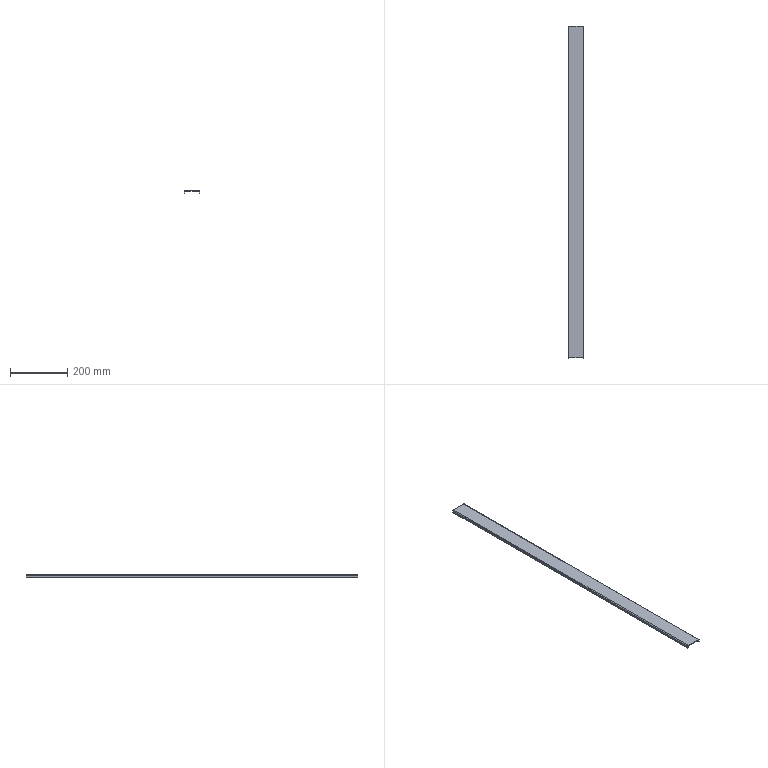Part | SolidWorks | features BaseBody 1 | 1 solid | 22 faces | box 56 x 1162 x 10 mm | volume 201891 mm3 | plane 18 | cylinder 4 | commonest cylinder face diameters 1 x2 6 x2
STEP:
#1=CARTESIAN_POINT('',(-25.5,581.,-10.));
#2=VERTEX_POINT('',#1);
#3=CARTESIAN_POINT('',(-25.5,-581.,-10.));
#4=VERTEX_POINT('',#3);
#5=CARTESIAN_POINT('',(-25.5,-581.,-10.));
#6=DIRECTION('',(0.,-1.,0.));
#7=VECTOR('',#6,1000.);
#8=LINE('',#5,#7);
#9=EDGE_CURVE('',#2,#4,#8,.T.);
#10=ORIENTED_EDGE('',*,*,#9,.T.);
#11=CARTESIAN_POINT('',(-28.,-581.,-10.));
#12=VERTEX_POINT('',#11);
#13=CARTESIAN_POINT('',(-28.,-581.,-10.));
#14=DIRECTION('',(1.,0.,0.));
#15=VECTOR('',#14,1000.);
#16=LINE('',#13,#15);
#17=EDGE_CURVE('',#12,#4,#16,.T.);
#18=ORIENTED_EDGE('',*,*,#17,.F.);
#19=CARTESIAN_POINT('',(-28.,581.,-10.));
#20=VERTEX_POINT('',#19);
#21=CARTESIAN_POINT('',(-28.,0.,-10.));
#22=DIRECTION('',(0.,-1.,0.));
#23=VECTOR('',#22,1000.);
#24=LINE('',#21,#23);
#25=EDGE_CURVE('',#20,#12,#24,.T.);
#26=ORIENTED_EDGE('',*,*,#25,.F.);
#27=CARTESIAN_POINT('',(-28.,581.,-10.));
#28=DIRECTION('',(1.,0.,0.));
#29=VECTOR('',#28,1000.);
#30=LINE('',#27,#29);
#31=EDGE_CURVE('',#20,#2,#30,.T.);
#32=ORIENTED_EDGE('',*,*,#31,.T.);
#33=EDGE_LOOP('',(#10,#18,#26,#32));
#34=FACE_OUTER_BOUND('',#33,.T.);
#35=CARTESIAN_POINT('',(-28.,-581.,-10.));
#36=DIRECTION('',(0.,0.,1.));
#37=DIRECTION('',(1.,0.,0.));
#38=AXIS2_PLACEMENT_3D('',#35,#36,#37);
#39=PLANE('',#38);
#40=ADVANCED_FACE('',(#34),#39,.F.);
#41=CARTESIAN_POINT('',(-25.5,581.,-3.));
#42=VERTEX_POINT('',#41);
#43=CARTESIAN_POINT('',(-25.5,581.,-10.));
#44=DIRECTION('',(0.,0.,-1.));
#45=VECTOR('',#44,1000.);
#46=LINE('',#43,#45);
#47=EDGE_CURVE('',#42,#2,#46,.T.);
#48=ORIENTED_EDGE('',*,*,#47,.F.);
#49=CARTESIAN_POINT('',(-25.5,-581.,-3.));
#50=VERTEX_POINT('',#49);
#51=CARTESIAN_POINT('',(-25.5,-581.,-3.));
#52=DIRECTION('',(0.,1.,0.));
#53=VECTOR('',#52,1000.);
#54=LINE('',#51,#53);
#55=EDGE_CURVE('',#50,#42,#54,.T.);
#56=ORIENTED_EDGE('',*,*,#55,.F.);
#57=CARTESIAN_POINT('',(-25.5,-581.,-2.5));
#58=DIRECTION('',(0.,0.,1.));
#59=VECTOR('',#58,1000.);
#60=LINE('',#57,#59);
#61=EDGE_CURVE('',#4,#50,#60,.T.);
#62=ORIENTED_EDGE('',*,*,#61,.F.);
#63=ORIENTED_EDGE('',*,*,#9,.F.);
#64=EDGE_LOOP('',(#48,#56,#62,#63));
#65=FACE_OUTER_BOUND('',#64,.T.);
#66=CARTESIAN_POINT('',(-25.5,0.,0.));
#67=DIRECTION('',(1.,0.,0.));
#68=DIRECTION('',(0.,0.,-1.));
#69=AXIS2_PLACEMENT_3D('',#66,#67,#68);
#70=PLANE('',#69);
#71=ADVANCED_FACE('',(#65),#70,.T.);
#72=CARTESIAN_POINT('',(-28.,581.,-3.));
#73=VERTEX_POINT('',#72);
#74=CARTESIAN_POINT('',(-28.,-581.,-3.));
#75=VERTEX_POINT('',#74);
#76=CARTESIAN_POINT('',(-28.,-581.,-3.));
#77=DIRECTION('',(0.,-1.,0.));
#78=VECTOR('',#77,1000.);
#79=LINE('',#76,#78);
#80=EDGE_CURVE('',#73,#75,#79,.T.);
#81=ORIENTED_EDGE('',*,*,#80,.F.);
#82=CARTESIAN_POINT('',(-28.,581.,0.));
#83=DIRECTION('',(0.,0.,-1.));
#84=VECTOR('',#83,1000.);
#85=LINE('',#82,#84);
#86=EDGE_CURVE('',#73,#20,#85,.T.);
#87=ORIENTED_EDGE('',*,*,#86,.T.);
#88=ORIENTED_EDGE('',*,*,#25,.T.);
#89=CARTESIAN_POINT('',(-28.,-581.,0.));
#90=DIRECTION('',(0.,0.,1.));
#91=VECTOR('',#90,1000.);
#92=LINE('',#89,#91);
#93=EDGE_CURVE('',#12,#75,#92,.T.);
#94=ORIENTED_EDGE('',*,*,#93,.T.);
#95=EDGE_LOOP('',(#81,#87,#88,#94));
#96=FACE_OUTER_BOUND('',#95,.T.);
#97=CARTESIAN_POINT('',(-28.,0.,0.));
#98=DIRECTION('',(1.,0.,0.));
#99=DIRECTION('',(0.,0.,-1.));
#100=AXIS2_PLACEMENT_3D('',#97,#98,#99);
#101=PLANE('',#100);
#102=ADVANCED_FACE('',(#96),#101,.F.);
#103=CARTESIAN_POINT('',(-28.,-581.,-3.));
#104=DIRECTION('',(-1.,0.,0.));
#105=VECTOR('',#104,1000.);
#106=LINE('',#103,#105);
#107=EDGE_CURVE('',#50,#75,#106,.T.);
#108=ORIENTED_EDGE('',*,*,#107,.T.);
#109=ORIENTED_EDGE('',*,*,#93,.F.);
#110=ORIENTED_EDGE('',*,*,#17,.T.);
#111=ORIENTED_EDGE('',*,*,#61,.T.);
#112=EDGE_LOOP('',(#108,#109,#110,#111));
#113=FACE_OUTER_BOUND('',#112,.T.);
#114=CARTESIAN_POINT('',(-28.,-581.,-2.5));
#115=DIRECTION('',(0.,1.,0.));
#116=DIRECTION('',(1.,0.,0.));
#117=AXIS2_PLACEMENT_3D('',#114,#115,#116);
#118=PLANE('',#117);
#119=ADVANCED_FACE('',(#113),#118,.F.);
#120=CARTESIAN_POINT('',(-25.5,581.,-3.));
#121=DIRECTION('',(-1.,0.,0.));
#122=VECTOR('',#121,1000.);
#123=LINE('',#120,#122);
#124=EDGE_CURVE('',#42,#73,#123,.T.);
#125=ORIENTED_EDGE('',*,*,#124,.F.);
#126=ORIENTED_EDGE('',*,*,#47,.T.);
#127=ORIENTED_EDGE('',*,*,#31,.F.);
#128=ORIENTED_EDGE('',*,*,#86,.F.);
#129=EDGE_LOOP('',(#125,#126,#127,#128));
#130=FACE_OUTER_BOUND('',#129,.T.);
#131=CARTESIAN_POINT('',(-28.,581.,-10.));
#132=DIRECTION('',(0.,-1.,0.));
#133=DIRECTION('',(0.,0.,-1.));
#134=AXIS2_PLACEMENT_3D('',#131,#132,#133);
#135=PLANE('',#134);
#136=ADVANCED_FACE('',(#130),#135,.F.);
#137=CARTESIAN_POINT('',(-25.,581.,-2.5));
#138=VERTEX_POINT('',#137);
#139=CARTESIAN_POINT('',(-25.,-581.,-2.5));
#140=VERTEX_POINT('',#139);
#141=CARTESIAN_POINT('',(-25.,581.,-2.5));
#142=DIRECTION('',(0.,-1.,0.));
#143=VECTOR('',#142,1000.);
#144=LINE('',#141,#143);
#145=EDGE_CURVE('',#138,#140,#144,.T.);
#146=ORIENTED_EDGE('',*,*,#145,.T.);
#147=CARTESIAN_POINT('',(-25.,-581.,-3.));
#148=DIRECTION('',(0.,-1.,0.));
#149=DIRECTION('',(0.,0.,1.));
#150=AXIS2_PLACEMENT_3D('',#147,#148,#149);
#151=CIRCLE('',#150,0.5);
#152=EDGE_CURVE('',#140,#50,#151,.T.);
#153=ORIENTED_EDGE('',*,*,#152,.T.);
#154=ORIENTED_EDGE('',*,*,#55,.T.);
#155=CARTESIAN_POINT('',(-25.,581.,-3.));
#156=DIRECTION('',(0.,1.,0.));
#157=DIRECTION('',(0.,0.,1.));
#158=AXIS2_PLACEMENT_3D('',#155,#156,#157);
#159=CIRCLE('',#158,0.5);
#160=EDGE_CURVE('',#42,#138,#159,.T.);
#161=ORIENTED_EDGE('',*,*,#160,.T.);
#162=EDGE_LOOP('',(#146,#153,#154,#161));
#163=FACE_OUTER_BOUND('',#162,.T.);
#164=CARTESIAN_POINT('',(-25.,581.,-3.));
#165=DIRECTION('',(0.,1.,0.));
#166=DIRECTION('',(-1.,0.,0.));
#167=AXIS2_PLACEMENT_3D('',#164,#165,#166);
#168=CYLINDRICAL_SURFACE('',#167,0.5);
#169=ADVANCED_FACE('',(#163),#168,.F.);
#170=CARTESIAN_POINT('',(-25.,581.,0.));
#171=VERTEX_POINT('',#170);
#172=CARTESIAN_POINT('',(-25.,-581.,0.));
#173=VERTEX_POINT('',#172);
#174=CARTESIAN_POINT('',(-25.,581.,0.));
#175=DIRECTION('',(0.,-1.,0.));
#176=VECTOR('',#175,1000.);
#177=LINE('',#174,#176);
#178=EDGE_CURVE('',#171,#173,#177,.T.);
#179=ORIENTED_EDGE('',*,*,#178,.F.);
#180=CARTESIAN_POINT('',(-25.,581.,-3.));
#181=DIRECTION('',(0.,1.,0.));
#182=DIRECTION('',(0.,0.,1.));
#183=AXIS2_PLACEMENT_3D('',#180,#181,#182);
#184=CIRCLE('',#183,3.);
#185=EDGE_CURVE('',#73,#171,#184,.T.);
#186=ORIENTED_EDGE('',*,*,#185,.F.);
#187=ORIENTED_EDGE('',*,*,#80,.T.);
#188=CARTESIAN_POINT('',(-25.,-581.,-3.));
#189=DIRECTION('',(0.,-1.,0.));
#190=DIRECTION('',(0.,0.,1.));
#191=AXIS2_PLACEMENT_3D('',#188,#189,#190);
#192=CIRCLE('',#191,3.);
#193=EDGE_CURVE('',#173,#75,#192,.T.);
#194=ORIENTED_EDGE('',*,*,#193,.F.);
#195=EDGE_LOOP('',(#179,#186,#187,#194));
#196=FACE_OUTER_BOUND('',#195,.T.);
#197=CARTESIAN_POINT('',(-25.,581.,-3.));
#198=DIRECTION('',(0.,1.,0.));
#199=DIRECTION('',(-1.,0.,0.));
#200=AXIS2_PLACEMENT_3D('',#197,#198,#199);
#201=CYLINDRICAL_SURFACE('',#200,3.);
#202=ADVANCED_FACE('',(#196),#201,.T.);
#203=ORIENTED_EDGE('',*,*,#160,.F.);
#204=ORIENTED_EDGE('',*,*,#124,.T.);
#205=ORIENTED_EDGE('',*,*,#185,.T.);
#206=CARTESIAN_POINT('',(-25.,581.,-2.5));
#207=DIRECTION('',(0.,0.,1.));
#208=VECTOR('',#207,1000.);
#209=LINE('',#206,#208);
#210=EDGE_CURVE('',#138,#171,#209,.T.);
#211=ORIENTED_EDGE('',*,*,#210,.F.);
#212=EDGE_LOOP('',(#203,#204,#205,#211));
#213=FACE_OUTER_BOUND('',#212,.T.);
#214=CARTESIAN_POINT('',(-25.,581.,-3.));
#215=DIRECTION('',(0.,-1.,0.));
#216=DIRECTION('',(0.,0.,-1.));
#217=AXIS2_PLACEMENT_3D('',#214,#215,#216);
#218=PLANE('',#217);
#219=ADVANCED_FACE('',(#213),#218,.F.);
#220=ORIENTED_EDGE('',*,*,#107,.F.);
#221=ORIENTED_EDGE('',*,*,#152,.F.);
#222=CARTESIAN_POINT('',(-25.,-581.,-2.5));
#223=DIRECTION('',(0.,0.,1.));
#224=VECTOR('',#223,1000.);
#225=LINE('',#222,#224);
#226=EDGE_CURVE('',#140,#173,#225,.T.);
#227=ORIENTED_EDGE('',*,*,#226,.T.);
#228=ORIENTED_EDGE('',*,*,#193,.T.);
#229=EDGE_LOOP('',(#220,#221,#227,#228));
#230=FACE_OUTER_BOUND('',#229,.T.);
#231=CARTESIAN_POINT('',(-25.,-581.,-3.));
#232=DIRECTION('',(0.,-1.,0.));
#233=DIRECTION('',(0.,0.,-1.));
#234=AXIS2_PLACEMENT_3D('',#231,#232,#233);
#235=PLANE('',#234);
#236=ADVANCED_FACE('',(#230),#235,.T.);
#237=CARTESIAN_POINT('',(25.5,-581.,-10.));
#238=VERTEX_POINT('',#237);
#239=CARTESIAN_POINT('',(25.5,581.,-10.));
#240=VERTEX_POINT('',#239);
#241=CARTESIAN_POINT('',(25.5,581.,-10.));
#242=DIRECTION('',(0.,1.,0.));
#243=VECTOR('',#242,1000.);
#244=LINE('',#241,#243);
#245=EDGE_CURVE('',#238,#240,#244,.T.);
#246=ORIENTED_EDGE('',*,*,#245,.T.);
#247=CARTESIAN_POINT('',(28.,581.,-10.));
#248=VERTEX_POINT('',#247);
#249=CARTESIAN_POINT('',(28.,581.,-10.));
#250=DIRECTION('',(-1.,0.,0.));
#251=VECTOR('',#250,1000.);
#252=LINE('',#249,#251);
#253=EDGE_CURVE('',#248,#240,#252,.T.);
#254=ORIENTED_EDGE('',*,*,#253,.F.);
#255=CARTESIAN_POINT('',(28.,-581.,-10.));
#256=VERTEX_POINT('',#255);
#257=CARTESIAN_POINT('',(28.,0.,-10.));
#258=DIRECTION('',(0.,1.,0.));
#259=VECTOR('',#258,1000.);
#260=LINE('',#257,#259);
#261=EDGE_CURVE('',#256,#248,#260,.T.);
#262=ORIENTED_EDGE('',*,*,#261,.F.);
#263=CARTESIAN_POINT('',(28.,-581.,-10.));
#264=DIRECTION('',(-1.,0.,0.));
#265=VECTOR('',#264,1000.);
#266=LINE('',#263,#265);
#267=EDGE_CURVE('',#256,#238,#266,.T.);
#268=ORIENTED_EDGE('',*,*,#267,.T.);
#269=EDGE_LOOP('',(#246,#254,#262,#268));
#270=FACE_OUTER_BOUND('',#269,.T.);
#271=CARTESIAN_POINT('',(28.,581.,-10.));
#272=DIRECTION('',(0.,0.,1.));
#273=DIRECTION('',(1.,0.,0.));
#274=AXIS2_PLACEMENT_3D('',#271,#272,#273);
#275=PLANE('',#274);
#276=ADVANCED_FACE('',(#270),#275,.F.);
#277=CARTESIAN_POINT('',(25.5,-581.,-3.));
#278=VERTEX_POINT('',#277);
#279=CARTESIAN_POINT('',(25.5,-581.,-10.));
#280=DIRECTION('',(0.,0.,-1.));
#281=VECTOR('',#280,1000.);
#282=LINE('',#279,#281);
#283=EDGE_CURVE('',#278,#238,#282,.T.);
#284=ORIENTED_EDGE('',*,*,#283,.F.);
#285=CARTESIAN_POINT('',(25.5,581.,-3.));
#286=VERTEX_POINT('',#285);
#287=CARTESIAN_POINT('',(25.5,581.,-3.));
#288=DIRECTION('',(0.,-1.,0.));
#289=VECTOR('',#288,1000.);
#290=LINE('',#287,#289);
#291=EDGE_CURVE('',#286,#278,#290,.T.);
#292=ORIENTED_EDGE('',*,*,#291,.F.);
#293=CARTESIAN_POINT('',(25.5,581.,-2.5));
#294=DIRECTION('',(0.,0.,1.));
#295=VECTOR('',#294,1000.);
#296=LINE('',#293,#295);
#297=EDGE_CURVE('',#240,#286,#296,.T.);
#298=ORIENTED_EDGE('',*,*,#297,.F.);
#299=ORIENTED_EDGE('',*,*,#245,.F.);
#300=EDGE_LOOP('',(#284,#292,#298,#299));
#301=FACE_OUTER_BOUND('',#300,.T.);
#302=CARTESIAN_POINT('',(25.5,0.,0.));
#303=DIRECTION('',(-1.,0.,0.));
#304=DIRECTION('',(0.,0.,1.));
#305=AXIS2_PLACEMENT_3D('',#302,#303,#304);
#306=PLANE('',#305);
#307=ADVANCED_FACE('',(#301),#306,.T.);
#308=CARTESIAN_POINT('',(28.,-581.,-3.));
#309=VERTEX_POINT('',#308);
#310=CARTESIAN_POINT('',(28.,581.,-3.));
#311=VERTEX_POINT('',#310);
#312=CARTESIAN_POINT('',(28.,581.,-3.));
#313=DIRECTION('',(0.,1.,0.));
#314=VECTOR('',#313,1000.);
#315=LINE('',#312,#314);
#316=EDGE_CURVE('',#309,#311,#315,.T.);
#317=ORIENTED_EDGE('',*,*,#316,.F.);
#318=CARTESIAN_POINT('',(28.,-581.,0.));
#319=DIRECTION('',(0.,0.,-1.));
#320=VECTOR('',#319,1000.);
#321=LINE('',#318,#320);
#322=EDGE_CURVE('',#309,#256,#321,.T.);
#323=ORIENTED_EDGE('',*,*,#322,.T.);
#324=ORIENTED_EDGE('',*,*,#261,.T.);
#325=CARTESIAN_POINT('',(28.,581.,0.));
#326=DIRECTION('',(0.,0.,1.));
#327=VECTOR('',#326,1000.);
#328=LINE('',#325,#327);
#329=EDGE_CURVE('',#248,#311,#328,.T.);
#330=ORIENTED_EDGE('',*,*,#329,.T.);
#331=EDGE_LOOP('',(#317,#323,#324,#330));
#332=FACE_OUTER_BOUND('',#331,.T.);
#333=CARTESIAN_POINT('',(28.,0.,0.));
#334=DIRECTION('',(-1.,0.,0.));
#335=DIRECTION('',(0.,0.,1.));
#336=AXIS2_PLACEMENT_3D('',#333,#334,#335);
#337=PLANE('',#336);
#338=ADVANCED_FACE('',(#332),#337,.F.);
#339=CARTESIAN_POINT('',(28.,581.,-3.));
#340=DIRECTION('',(1.,0.,0.));
#341=VECTOR('',#340,1000.);
#342=LINE('',#339,#341);
#343=EDGE_CURVE('',#286,#311,#342,.T.);
#344=ORIENTED_EDGE('',*,*,#343,.T.);
#345=ORIENTED_EDGE('',*,*,#329,.F.);
#346=ORIENTED_EDGE('',*,*,#253,.T.);
#347=ORIENTED_EDGE('',*,*,#297,.T.);
#348=EDGE_LOOP('',(#344,#345,#346,#347));
#349=FACE_OUTER_BOUND('',#348,.T.);
#350=CARTESIAN_POINT('',(28.,581.,-2.5));
#351=DIRECTION('',(0.,-1.,0.));
#352=DIRECTION('',(0.,0.,-1.));
#353=AXIS2_PLACEMENT_3D('',#350,#351,#352);
#354=PLANE('',#353);
#355=ADVANCED_FACE('',(#349),#354,.F.);
#356=CARTESIAN_POINT('',(25.5,-581.,-3.));
#357=DIRECTION('',(1.,0.,0.));
#358=VECTOR('',#357,1000.);
#359=LINE('',#356,#358);
#360=EDGE_CURVE('',#278,#309,#359,.T.);
#361=ORIENTED_EDGE('',*,*,#360,.F.);
#362=ORIENTED_EDGE('',*,*,#283,.T.);
#363=ORIENTED_EDGE('',*,*,#267,.F.);
#364=ORIENTED_EDGE('',*,*,#322,.F.);
#365=EDGE_LOOP('',(#361,#362,#363,#364));
#366=FACE_OUTER_BOUND('',#365,.T.);
#367=CARTESIAN_POINT('',(28.,-581.,-10.));
#368=DIRECTION('',(0.,1.,0.));
#369=DIRECTION('',(1.,0.,0.));
#370=AXIS2_PLACEMENT_3D('',#367,#368,#369);
#371=PLANE('',#370);
#372=ADVANCED_FACE('',(#366),#371,.F.);
#373=CARTESIAN_POINT('',(25.,-581.,-2.5));
#374=VERTEX_POINT('',#373);
#375=CARTESIAN_POINT('',(25.,581.,-2.5));
#376=VERTEX_POINT('',#375);
#377=CARTESIAN_POINT('',(25.,-581.,-2.5));
#378=DIRECTION('',(0.,1.,0.));
#379=VECTOR('',#378,1000.);
#380=LINE('',#377,#379);
#381=EDGE_CURVE('',#374,#376,#380,.T.);
#382=ORIENTED_EDGE('',*,*,#381,.T.);
#383=CARTESIAN_POINT('',(25.,581.,-3.));
#384=DIRECTION('',(0.,1.,0.));
#385=DIRECTION('',(0.,0.,-1.));
#386=AXIS2_PLACEMENT_3D('',#383,#384,#385);
#387=CIRCLE('',#386,0.5);
#388=EDGE_CURVE('',#376,#286,#387,.T.);
#389=ORIENTED_EDGE('',*,*,#388,.T.);
#390=ORIENTED_EDGE('',*,*,#291,.T.);
#391=CARTESIAN_POINT('',(25.,-581.,-3.));
#392=DIRECTION('',(0.,-1.,0.));
#393=DIRECTION('',(0.,0.,-1.));
#394=AXIS2_PLACEMENT_3D('',#391,#392,#393);
#395=CIRCLE('',#394,0.5);
#396=EDGE_CURVE('',#278,#374,#395,.T.);
#397=ORIENTED_EDGE('',*,*,#396,.T.);
#398=EDGE_LOOP('',(#382,#389,#390,#397));
#399=FACE_OUTER_BOUND('',#398,.T.);
#400=CARTESIAN_POINT('',(25.,-581.,-3.));
#401=DIRECTION('',(0.,-1.,0.));
#402=DIRECTION('',(1.,0.,0.));
#403=AXIS2_PLACEMENT_3D('',#400,#401,#402);
#404=CYLINDRICAL_SURFACE('',#403,0.5);
#405=ADVANCED_FACE('',(#399),#404,.F.);
#406=CARTESIAN_POINT('',(25.,-581.,0.));
#407=VERTEX_POINT('',#406);
#408=CARTESIAN_POINT('',(25.,581.,0.));
#409=VERTEX_POINT('',#408);
#410=CARTESIAN_POINT('',(25.,-581.,0.));
#411=DIRECTION('',(0.,1.,0.));
#412=VECTOR('',#411,1000.);
#413=LINE('',#410,#412);
#414=EDGE_CURVE('',#407,#409,#413,.T.);
#415=ORIENTED_EDGE('',*,*,#414,.F.);
#416=CARTESIAN_POINT('',(25.,-581.,-3.));
#417=DIRECTION('',(0.,-1.,0.));
#418=DIRECTION('',(0.,0.,-1.));
#419=AXIS2_PLACEMENT_3D('',#416,#417,#418);
#420=CIRCLE('',#419,3.);
#421=EDGE_CURVE('',#309,#407,#420,.T.);
#422=ORIENTED_EDGE('',*,*,#421,.F.);
#423=ORIENTED_EDGE('',*,*,#316,.T.);
#424=CARTESIAN_POINT('',(25.,581.,-3.));
#425=DIRECTION('',(0.,1.,0.));
#426=DIRECTION('',(0.,0.,-1.));
#427=AXIS2_PLACEMENT_3D('',#424,#425,#426);
#428=CIRCLE('',#427,3.);
#429=EDGE_CURVE('',#409,#311,#428,.T.);
#430=ORIENTED_EDGE('',*,*,#429,.F.);
#431=EDGE_LOOP('',(#415,#422,#423,#430));
#432=FACE_OUTER_BOUND('',#431,.T.);
#433=CARTESIAN_POINT('',(25.,-581.,-3.));
#434=DIRECTION('',(0.,-1.,0.));
#435=DIRECTION('',(1.,0.,0.));
#436=AXIS2_PLACEMENT_3D('',#433,#434,#435);
#437=CYLINDRICAL_SURFACE('',#436,3.);
#438=ADVANCED_FACE('',(#432),#437,.T.);
#439=ORIENTED_EDGE('',*,*,#396,.F.);
#440=ORIENTED_EDGE('',*,*,#360,.T.);
#441=ORIENTED_EDGE('',*,*,#421,.T.);
#442=CARTESIAN_POINT('',(25.,-581.,-2.5));
#443=DIRECTION('',(0.,0.,1.));
#444=VECTOR('',#443,1000.);
#445=LINE('',#442,#444);
#446=EDGE_CURVE('',#374,#407,#445,.T.);
#447=ORIENTED_EDGE('',*,*,#446,.F.);
#448=EDGE_LOOP('',(#439,#440,#441,#447));
#449=FACE_OUTER_BOUND('',#448,.T.);
#450=CARTESIAN_POINT('',(25.,-581.,-3.));
#451=DIRECTION('',(0.,1.,0.));
#452=DIRECTION('',(1.,0.,0.));
#453=AXIS2_PLACEMENT_3D('',#450,#451,#452);
#454=PLANE('',#453);
#455=ADVANCED_FACE('',(#449),#454,.F.);
#456=ORIENTED_EDGE('',*,*,#343,.F.);
#457=ORIENTED_EDGE('',*,*,#388,.F.);
#458=CARTESIAN_POINT('',(25.,581.,-2.5));
#459=DIRECTION('',(0.,0.,1.));
#460=VECTOR('',#459,1000.);
#461=LINE('',#458,#460);
#462=EDGE_CURVE('',#376,#409,#461,.T.);
#463=ORIENTED_EDGE('',*,*,#462,.T.);
#464=ORIENTED_EDGE('',*,*,#429,.T.);
#465=EDGE_LOOP('',(#456,#457,#463,#464));
#466=FACE_OUTER_BOUND('',#465,.T.);
#467=CARTESIAN_POINT('',(25.,581.,-3.));
#468=DIRECTION('',(0.,1.,0.));
#469=DIRECTION('',(1.,0.,0.));
#470=AXIS2_PLACEMENT_3D('',#467,#468,#469);
#471=PLANE('',#470);
#472=ADVANCED_FACE('',(#466),#471,.T.);
#473=ORIENTED_EDGE('',*,*,#226,.F.);
#474=CARTESIAN_POINT('',(28.,-581.,-2.5));
#475=DIRECTION('',(1.,0.,0.));
#476=VECTOR('',#475,1000.);
#477=LINE('',#474,#476);
#478=EDGE_CURVE('',#140,#374,#477,.T.);
#479=ORIENTED_EDGE('',*,*,#478,.T.);
#480=ORIENTED_EDGE('',*,*,#446,.T.);
#481=CARTESIAN_POINT('',(28.,-581.,0.));
#482=DIRECTION('',(1.,0.,0.));
#483=VECTOR('',#482,1000.);
#484=LINE('',#481,#483);
#485=EDGE_CURVE('',#173,#407,#484,.T.);
#486=ORIENTED_EDGE('',*,*,#485,.F.);
#487=EDGE_LOOP('',(#473,#479,#480,#486));
#488=FACE_OUTER_BOUND('',#487,.T.);
#489=CARTESIAN_POINT('',(28.,-581.,-2.5));
#490=DIRECTION('',(0.,-1.,0.));
#491=DIRECTION('',(0.,0.,-1.));
#492=AXIS2_PLACEMENT_3D('',#489,#490,#491);
#493=PLANE('',#492);
#494=ADVANCED_FACE('',(#488),#493,.T.);
#495=CARTESIAN_POINT('',(28.,581.,-2.5));
#496=DIRECTION('',(-1.,0.,0.));
#497=VECTOR('',#496,1000.);
#498=LINE('',#495,#497);
#499=EDGE_CURVE('',#376,#138,#498,.T.);
#500=ORIENTED_EDGE('',*,*,#499,.T.);
#501=ORIENTED_EDGE('',*,*,#210,.T.);
#502=CARTESIAN_POINT('',(28.,581.,0.));
#503=DIRECTION('',(-1.,0.,0.));
#504=VECTOR('',#503,1000.);
#505=LINE('',#502,#504);
#506=EDGE_CURVE('',#409,#171,#505,.T.);
#507=ORIENTED_EDGE('',*,*,#506,.F.);
#508=ORIENTED_EDGE('',*,*,#462,.F.);
#509=EDGE_LOOP('',(#500,#501,#507,#508));
#510=FACE_OUTER_BOUND('',#509,.T.);
#511=CARTESIAN_POINT('',(28.,581.,-2.5));
#512=DIRECTION('',(0.,1.,0.));
#513=DIRECTION('',(1.,0.,0.));
#514=AXIS2_PLACEMENT_3D('',#511,#512,#513);
#515=PLANE('',#514);
#516=ADVANCED_FACE('',(#510),#515,.T.);
#517=ORIENTED_EDGE('',*,*,#178,.T.);
#518=ORIENTED_EDGE('',*,*,#485,.T.);
#519=ORIENTED_EDGE('',*,*,#414,.T.);
#520=ORIENTED_EDGE('',*,*,#506,.T.);
#521=EDGE_LOOP('',(#517,#518,#519,#520));
#522=FACE_OUTER_BOUND('',#521,.T.);
#523=CARTESIAN_POINT('',(0.,0.,0.));
#524=DIRECTION('',(0.,0.,-1.));
#525=DIRECTION('',(0.,-1.,0.));
#526=AXIS2_PLACEMENT_3D('',#523,#524,#525);
#527=PLANE('',#526);
#528=ADVANCED_FACE('',(#522),#527,.F.);
#529=ORIENTED_EDGE('',*,*,#478,.F.);
#530=ORIENTED_EDGE('',*,*,#145,.F.);
#531=ORIENTED_EDGE('',*,*,#499,.F.);
#532=ORIENTED_EDGE('',*,*,#381,.F.);
#533=EDGE_LOOP('',(#529,#530,#531,#532));
#534=FACE_OUTER_BOUND('',#533,.T.);
#535=CARTESIAN_POINT('',(0.,0.,-2.5));
#536=DIRECTION('',(0.,0.,-1.));
#537=DIRECTION('',(0.,-1.,0.));
#538=AXIS2_PLACEMENT_3D('',#535,#536,#537);
#539=PLANE('',#538);
#540=ADVANCED_FACE('',(#534),#539,.T.);
#541=CLOSED_SHELL('',(#40,#71,#102,#119,#136,#169,#202,#219,#236,#276,#307,#338,#355,#372,#405,#438,#455,#472,#494,#516,#528,#540));
#542=MANIFOLD_SOLID_BREP('',#541);
#543=CARTESIAN_POINT('',(0.,0.,0.));
#544=DIRECTION('',(0.,0.,1.));
#545=DIRECTION('',(1.,0.,0.));
#546=AXIS2_PLACEMENT_3D('',#543,#544,#545);
#547=(LENGTH_UNIT()NAMED_UNIT(*)SI_UNIT(.MILLI.,.METRE.));
#548=UNCERTAINTY_MEASURE_WITH_UNIT(LENGTH_MEASURE(0.00001),#547,'','');
#549=(NAMED_UNIT(*)PLANE_ANGLE_UNIT()SI_UNIT($,.RADIAN.));
#550=(NAMED_UNIT(*)SI_UNIT($,.STERADIAN.)SOLID_ANGLE_UNIT());
#551=(GEOMETRIC_REPRESENTATION_CONTEXT(3)GLOBAL_UNCERTAINTY_ASSIGNED_CONTEXT((#548))GLOBAL_UNIT_ASSIGNED_CONTEXT((#547,#549,#550))REPRESENTATION_CONTEXT('',''));
#552=ADVANCED_BREP_SHAPE_REPRESENTATION('',(#542,#546),#551);